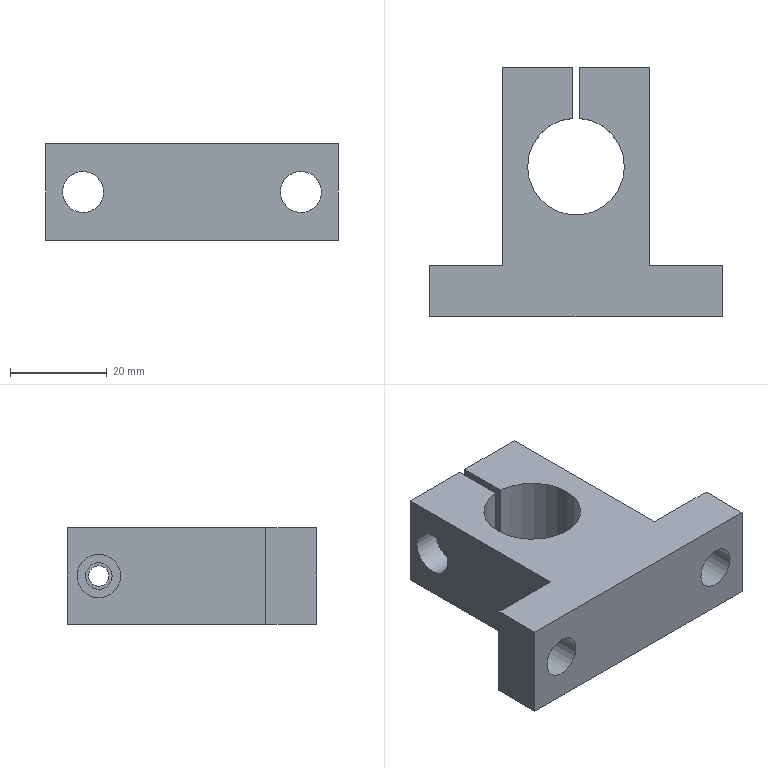Part | STEP file | 20310 | 1 solid | 27 faces | box 60.5 x 51.5 x 20 mm | volume 29160 mm3 | plane 14 | cylinder 13 | commonest cylinder face diameters 8.5 x4 20 x3 4.2 x2 5.5 x2 9 x2
STEP:
#1=CARTESIAN_POINT('',(-26.23,0.,7.962));
#2=VERTEX_POINT('',#1);
#3=CARTESIAN_POINT('',(-26.23,10.5,7.962));
#4=VERTEX_POINT('',#3);
#5=CARTESIAN_POINT('',(-26.23,13.155,7.962));
#6=DIRECTION('',(0.,-1.,0.));
#7=VECTOR('',#6,1.);
#8=LINE('',#5,#7);
#9=EDGE_CURVE('',#2,#4,#8,.F.);
#10=ORIENTED_EDGE('',*,*,#9,.F.);
#11=CARTESIAN_POINT('',(-18.77,0.,12.038));
#12=VERTEX_POINT('',#11);
#13=CARTESIAN_POINT('',(-22.5,0.,10.));
#14=DIRECTION('',(0.,-1.,0.));
#15=AXIS2_PLACEMENT_3D('',#13,#14,$);
#16=CIRCLE('',#15,4.25);
#17=EDGE_CURVE('',#12,#2,#16,.F.);
#18=ORIENTED_EDGE('',*,*,#17,.F.);
#19=CARTESIAN_POINT('',(-18.77,10.5,12.038));
#20=VERTEX_POINT('',#19);
#21=CARTESIAN_POINT('',(-18.77,13.155,12.038));
#22=DIRECTION('',(0.,-1.,0.));
#23=VECTOR('',#22,1.);
#24=LINE('',#21,#23);
#25=EDGE_CURVE('',#12,#20,#24,.F.);
#26=ORIENTED_EDGE('',*,*,#25,.T.);
#27=CARTESIAN_POINT('',(-22.5,10.5,10.));
#28=DIRECTION('',(0.,-1.,0.));
#29=AXIS2_PLACEMENT_3D('',#27,#28,$);
#30=CIRCLE('',#29,4.25);
#31=EDGE_CURVE('',#4,#20,#30,.T.);
#32=ORIENTED_EDGE('',*,*,#31,.F.);
#33=EDGE_LOOP('',(#10,#18,#26,#32));
#34=FACE_OUTER_BOUND('',#33,.T.);
#35=CARTESIAN_POINT('',(-22.5,10.4,10.));
#36=DIRECTION('',(0.,-1.,0.));
#37=DIRECTION('',(0.8776,0.,0.4794));
#38=AXIS2_PLACEMENT_3D('',#35,#36,#37);
#39=CYLINDRICAL_SURFACE('',#38,4.25);
#40=ADVANCED_FACE('',(#34),#39,.F.);
#41=ORIENTED_EDGE('',*,*,#25,.F.);
#42=CARTESIAN_POINT('',(-22.5,0.,10.));
#43=DIRECTION('',(0.,-1.,0.));
#44=AXIS2_PLACEMENT_3D('',#42,#43,$);
#45=CIRCLE('',#44,4.25);
#46=EDGE_CURVE('',#2,#12,#45,.F.);
#47=ORIENTED_EDGE('',*,*,#46,.F.);
#48=ORIENTED_EDGE('',*,*,#9,.T.);
#49=CARTESIAN_POINT('',(-22.5,10.5,10.));
#50=DIRECTION('',(0.,-1.,0.));
#51=AXIS2_PLACEMENT_3D('',#49,#50,$);
#52=CIRCLE('',#51,4.25);
#53=EDGE_CURVE('',#20,#4,#52,.T.);
#54=ORIENTED_EDGE('',*,*,#53,.F.);
#55=EDGE_LOOP('',(#41,#47,#48,#54));
#56=FACE_OUTER_BOUND('',#55,.T.);
#57=ADVANCED_FACE('',(#56),#39,.F.);
#58=CARTESIAN_POINT('',(-30.25,10.5,0.));
#59=VERTEX_POINT('',#58);
#60=CARTESIAN_POINT('',(-30.25,10.5,20.));
#61=VERTEX_POINT('',#60);
#62=CARTESIAN_POINT('',(-30.25,10.5,10.));
#63=DIRECTION('',(0.,0.,1.));
#64=VECTOR('',#63,1.);
#65=LINE('',#62,#64);
#66=EDGE_CURVE('',#59,#61,#65,.T.);
#67=ORIENTED_EDGE('',*,*,#66,.F.);
#68=CARTESIAN_POINT('',(-30.25,0.,0.));
#69=VERTEX_POINT('',#68);
#70=CARTESIAN_POINT('',(-30.25,5.25,0.));
#71=DIRECTION('',(0.,1.,0.));
#72=VECTOR('',#71,1.);
#73=LINE('',#70,#72);
#74=EDGE_CURVE('',#59,#69,#73,.F.);
#75=ORIENTED_EDGE('',*,*,#74,.T.);
#76=CARTESIAN_POINT('',(-30.25,0.,20.));
#77=VERTEX_POINT('',#76);
#78=CARTESIAN_POINT('',(-30.25,0.,10.));
#79=DIRECTION('',(0.,0.,1.));
#80=VECTOR('',#79,1.);
#81=LINE('',#78,#80);
#82=EDGE_CURVE('',#69,#77,#81,.T.);
#83=ORIENTED_EDGE('',*,*,#82,.T.);
#84=CARTESIAN_POINT('',(-30.25,5.25,20.));
#85=DIRECTION('',(0.,1.,0.));
#86=VECTOR('',#85,1.);
#87=LINE('',#84,#86);
#88=EDGE_CURVE('',#61,#77,#87,.F.);
#89=ORIENTED_EDGE('',*,*,#88,.F.);
#90=EDGE_LOOP('',(#67,#75,#83,#89));
#91=FACE_OUTER_BOUND('',#90,.T.);
#92=CARTESIAN_POINT('',(-30.25,0.,0.));
#93=DIRECTION('',(1.,0.,0.));
#94=DIRECTION('',(0.,1.,0.));
#95=AXIS2_PLACEMENT_3D('',#92,#93,#94);
#96=PLANE('',#95);
#97=ADVANCED_FACE('',(#91),#96,.F.);
#98=CARTESIAN_POINT('',(-0.75,51.5,0.));
#99=VERTEX_POINT('',#98);
#100=CARTESIAN_POINT('',(-0.75,40.972,0.));
#101=VERTEX_POINT('',#100);
#102=CARTESIAN_POINT('',(-0.75,46.236,0.));
#103=DIRECTION('',(0.,1.,0.));
#104=VECTOR('',#103,1.);
#105=LINE('',#102,#104);
#106=EDGE_CURVE('',#99,#101,#105,.F.);
#107=ORIENTED_EDGE('',*,*,#106,.T.);
#108=CARTESIAN_POINT('',(-10.,31.,0.));
#109=VERTEX_POINT('',#108);
#110=CARTESIAN_POINT('',(0.,31.,0.));
#111=DIRECTION('',(0.,0.,1.));
#112=AXIS2_PLACEMENT_3D('',#110,#111,$);
#113=CIRCLE('',#112,10.);
#114=EDGE_CURVE('',#101,#109,#113,.T.);
#115=ORIENTED_EDGE('',*,*,#114,.T.);
#116=CARTESIAN_POINT('',(10.,31.,0.));
#117=VERTEX_POINT('',#116);
#118=CARTESIAN_POINT('',(0.,31.,0.));
#119=DIRECTION('',(0.,0.,1.));
#120=AXIS2_PLACEMENT_3D('',#118,#119,$);
#121=CIRCLE('',#120,10.);
#122=EDGE_CURVE('',#109,#117,#121,.T.);
#123=ORIENTED_EDGE('',*,*,#122,.T.);
#124=CARTESIAN_POINT('',(0.75,40.972,0.));
#125=VERTEX_POINT('',#124);
#126=CARTESIAN_POINT('',(0.,31.,0.));
#127=DIRECTION('',(0.,0.,1.));
#128=AXIS2_PLACEMENT_3D('',#126,#127,$);
#129=CIRCLE('',#128,10.);
#130=EDGE_CURVE('',#117,#125,#129,.T.);
#131=ORIENTED_EDGE('',*,*,#130,.T.);
#132=CARTESIAN_POINT('',(0.75,51.5,0.));
#133=VERTEX_POINT('',#132);
#134=CARTESIAN_POINT('',(0.75,46.236,0.));
#135=DIRECTION('',(0.,-1.,0.));
#136=VECTOR('',#135,1.);
#137=LINE('',#134,#136);
#138=EDGE_CURVE('',#125,#133,#137,.F.);
#139=ORIENTED_EDGE('',*,*,#138,.T.);
#140=CARTESIAN_POINT('',(15.25,51.5,0.));
#141=VERTEX_POINT('',#140);
#142=CARTESIAN_POINT('',(8.,51.5,0.));
#143=DIRECTION('',(1.,0.,0.));
#144=VECTOR('',#143,1.);
#145=LINE('',#142,#144);
#146=EDGE_CURVE('',#141,#133,#145,.F.);
#147=ORIENTED_EDGE('',*,*,#146,.F.);
#148=CARTESIAN_POINT('',(15.25,10.5,0.));
#149=VERTEX_POINT('',#148);
#150=CARTESIAN_POINT('',(15.25,31.,0.));
#151=DIRECTION('',(0.,-1.,0.));
#152=VECTOR('',#151,1.);
#153=LINE('',#150,#152);
#154=EDGE_CURVE('',#149,#141,#153,.F.);
#155=ORIENTED_EDGE('',*,*,#154,.F.);
#156=CARTESIAN_POINT('',(30.25,10.5,0.));
#157=VERTEX_POINT('',#156);
#158=CARTESIAN_POINT('',(22.75,10.5,0.));
#159=DIRECTION('',(1.,0.,0.));
#160=VECTOR('',#159,1.);
#161=LINE('',#158,#160);
#162=EDGE_CURVE('',#157,#149,#161,.F.);
#163=ORIENTED_EDGE('',*,*,#162,.F.);
#164=CARTESIAN_POINT('',(30.25,0.,0.));
#165=VERTEX_POINT('',#164);
#166=CARTESIAN_POINT('',(30.25,5.25,0.));
#167=DIRECTION('',(0.,-1.,0.));
#168=VECTOR('',#167,1.);
#169=LINE('',#166,#168);
#170=EDGE_CURVE('',#165,#157,#169,.F.);
#171=ORIENTED_EDGE('',*,*,#170,.F.);
#172=CARTESIAN_POINT('',(0.,0.,0.));
#173=DIRECTION('',(-1.,0.,0.));
#174=VECTOR('',#173,1.);
#175=LINE('',#172,#174);
#176=EDGE_CURVE('',#69,#165,#175,.F.);
#177=ORIENTED_EDGE('',*,*,#176,.F.);
#178=ORIENTED_EDGE('',*,*,#74,.F.);
#179=CARTESIAN_POINT('',(-15.25,10.5,0.));
#180=VERTEX_POINT('',#179);
#181=CARTESIAN_POINT('',(-22.75,10.5,0.));
#182=DIRECTION('',(1.,0.,0.));
#183=VECTOR('',#182,1.);
#184=LINE('',#181,#183);
#185=EDGE_CURVE('',#180,#59,#184,.F.);
#186=ORIENTED_EDGE('',*,*,#185,.F.);
#187=CARTESIAN_POINT('',(-15.25,51.5,0.));
#188=VERTEX_POINT('',#187);
#189=CARTESIAN_POINT('',(-15.25,31.,0.));
#190=DIRECTION('',(0.,1.,0.));
#191=VECTOR('',#190,1.);
#192=LINE('',#189,#191);
#193=EDGE_CURVE('',#188,#180,#192,.F.);
#194=ORIENTED_EDGE('',*,*,#193,.F.);
#195=CARTESIAN_POINT('',(-8.,51.5,0.));
#196=DIRECTION('',(1.,0.,0.));
#197=VECTOR('',#196,1.);
#198=LINE('',#195,#197);
#199=EDGE_CURVE('',#99,#188,#198,.F.);
#200=ORIENTED_EDGE('',*,*,#199,.F.);
#201=EDGE_LOOP('',(#107,#115,#123,#131,#139,#147,#155,#163,#171,#177,#178,#186,#194,#200));
#202=FACE_OUTER_BOUND('',#201,.T.);
#203=CARTESIAN_POINT('',(0.,0.,0.));
#204=DIRECTION('',(0.,0.,1.));
#205=DIRECTION('',(1.,0.,0.));
#206=AXIS2_PLACEMENT_3D('',#203,#204,#205);
#207=PLANE('',#206);
#208=ADVANCED_FACE('',(#202),#207,.F.);
#209=ORIENTED_EDGE('',*,*,#138,.F.);
#210=CARTESIAN_POINT('',(0.75,40.972,20.));
#211=VERTEX_POINT('',#210);
#212=CARTESIAN_POINT('',(0.75,40.972,10.));
#213=DIRECTION('',(0.,0.,1.));
#214=VECTOR('',#213,1.);
#215=LINE('',#212,#214);
#216=EDGE_CURVE('',#125,#211,#215,.T.);
#217=ORIENTED_EDGE('',*,*,#216,.T.);
#218=CARTESIAN_POINT('',(0.75,51.5,20.));
#219=VERTEX_POINT('',#218);
#220=CARTESIAN_POINT('',(0.75,46.236,20.));
#221=DIRECTION('',(0.,-1.,0.));
#222=VECTOR('',#221,1.);
#223=LINE('',#220,#222);
#224=EDGE_CURVE('',#211,#219,#223,.F.);
#225=ORIENTED_EDGE('',*,*,#224,.T.);
#226=CARTESIAN_POINT('',(0.75,51.5,10.));
#227=DIRECTION('',(0.,0.,-1.));
#228=VECTOR('',#227,1.);
#229=LINE('',#226,#228);
#230=EDGE_CURVE('',#219,#133,#229,.T.);
#231=ORIENTED_EDGE('',*,*,#230,.T.);
#232=EDGE_LOOP('',(#209,#217,#225,#231));
#233=FACE_OUTER_BOUND('',#232,.T.);
#234=CARTESIAN_POINT('',(0.75,43.157,8.993));
#235=VERTEX_POINT('',#234);
#236=CARTESIAN_POINT('',(0.75,46.843,11.007));
#237=VERTEX_POINT('',#236);
#238=CARTESIAN_POINT('',(0.75,45.,10.));
#239=DIRECTION('',(1.,0.,0.));
#240=AXIS2_PLACEMENT_3D('',#238,#239,$);
#241=CIRCLE('',#240,2.1);
#242=EDGE_CURVE('',#235,#237,#241,.T.);
#243=ORIENTED_EDGE('',*,*,#242,.T.);
#244=CARTESIAN_POINT('',(0.75,45.,10.));
#245=DIRECTION('',(1.,0.,0.));
#246=AXIS2_PLACEMENT_3D('',#244,#245,$);
#247=CIRCLE('',#246,2.1);
#248=EDGE_CURVE('',#237,#235,#247,.T.);
#249=ORIENTED_EDGE('',*,*,#248,.T.);
#250=EDGE_LOOP('',(#243,#249));
#251=FACE_BOUND('',#250,.T.);
#252=CARTESIAN_POINT('',(0.75,60.,20.));
#253=DIRECTION('',(1.,0.,0.));
#254=DIRECTION('',(0.,-1.,0.));
#255=AXIS2_PLACEMENT_3D('',#252,#253,#254);
#256=PLANE('',#255);
#257=ADVANCED_FACE('',(#233,#251),#256,.F.);
#258=ORIENTED_EDGE('',*,*,#216,.F.);
#259=ORIENTED_EDGE('',*,*,#130,.F.);
#260=CARTESIAN_POINT('',(10.,31.,20.));
#261=VERTEX_POINT('',#260);
#262=CARTESIAN_POINT('',(10.,31.,10.));
#263=DIRECTION('',(0.,0.,1.));
#264=VECTOR('',#263,1.);
#265=LINE('',#262,#264);
#266=EDGE_CURVE('',#261,#117,#265,.F.);
#267=ORIENTED_EDGE('',*,*,#266,.F.);
#268=CARTESIAN_POINT('',(0.,31.,20.));
#269=DIRECTION('',(0.,0.,1.));
#270=AXIS2_PLACEMENT_3D('',#268,#269,$);
#271=CIRCLE('',#270,10.);
#272=EDGE_CURVE('',#261,#211,#271,.T.);
#273=ORIENTED_EDGE('',*,*,#272,.T.);
#274=EDGE_LOOP('',(#258,#259,#267,#273));
#275=FACE_OUTER_BOUND('',#274,.T.);
#276=CARTESIAN_POINT('',(0.,31.,10.));
#277=DIRECTION('',(0.,0.,1.));
#278=DIRECTION('',(1.,0.,0.));
#279=AXIS2_PLACEMENT_3D('',#276,#277,#278);
#280=CYLINDRICAL_SURFACE('',#279,10.);
#281=ADVANCED_FACE('',(#275),#280,.F.);
#282=CARTESIAN_POINT('',(-10.,31.,20.));
#283=VERTEX_POINT('',#282);
#284=CARTESIAN_POINT('',(-10.,31.,10.));
#285=DIRECTION('',(0.,0.,1.));
#286=VECTOR('',#285,1.);
#287=LINE('',#284,#286);
#288=EDGE_CURVE('',#283,#109,#287,.F.);
#289=ORIENTED_EDGE('',*,*,#288,.F.);
#290=CARTESIAN_POINT('',(0.,31.,20.));
#291=DIRECTION('',(0.,0.,1.));
#292=AXIS2_PLACEMENT_3D('',#290,#291,$);
#293=CIRCLE('',#292,10.);
#294=EDGE_CURVE('',#283,#261,#293,.T.);
#295=ORIENTED_EDGE('',*,*,#294,.T.);
#296=ORIENTED_EDGE('',*,*,#266,.T.);
#297=ORIENTED_EDGE('',*,*,#122,.F.);
#298=EDGE_LOOP('',(#289,#295,#296,#297));
#299=FACE_OUTER_BOUND('',#298,.T.);
#300=ADVANCED_FACE('',(#299),#280,.F.);
#301=CARTESIAN_POINT('',(-0.75,40.972,20.));
#302=VERTEX_POINT('',#301);
#303=CARTESIAN_POINT('',(-0.75,40.972,10.));
#304=DIRECTION('',(0.,0.,1.));
#305=VECTOR('',#304,1.);
#306=LINE('',#303,#305);
#307=EDGE_CURVE('',#101,#302,#306,.T.);
#308=ORIENTED_EDGE('',*,*,#307,.T.);
#309=CARTESIAN_POINT('',(0.,31.,20.));
#310=DIRECTION('',(0.,0.,1.));
#311=AXIS2_PLACEMENT_3D('',#309,#310,$);
#312=CIRCLE('',#311,10.);
#313=EDGE_CURVE('',#302,#283,#312,.T.);
#314=ORIENTED_EDGE('',*,*,#313,.T.);
#315=ORIENTED_EDGE('',*,*,#288,.T.);
#316=ORIENTED_EDGE('',*,*,#114,.F.);
#317=EDGE_LOOP('',(#308,#314,#315,#316));
#318=FACE_OUTER_BOUND('',#317,.T.);
#319=ADVANCED_FACE('',(#318),#280,.F.);
#320=ORIENTED_EDGE('',*,*,#106,.F.);
#321=CARTESIAN_POINT('',(-0.75,51.5,20.));
#322=VERTEX_POINT('',#321);
#323=CARTESIAN_POINT('',(-0.75,51.5,10.));
#324=DIRECTION('',(0.,0.,-1.));
#325=VECTOR('',#324,1.);
#326=LINE('',#323,#325);
#327=EDGE_CURVE('',#322,#99,#326,.T.);
#328=ORIENTED_EDGE('',*,*,#327,.F.);
#329=CARTESIAN_POINT('',(-0.75,46.236,20.));
#330=DIRECTION('',(0.,1.,0.));
#331=VECTOR('',#330,1.);
#332=LINE('',#329,#331);
#333=EDGE_CURVE('',#322,#302,#332,.F.);
#334=ORIENTED_EDGE('',*,*,#333,.T.);
#335=ORIENTED_EDGE('',*,*,#307,.F.);
#336=EDGE_LOOP('',(#320,#328,#334,#335));
#337=FACE_OUTER_BOUND('',#336,.T.);
#338=CARTESIAN_POINT('',(-0.75,42.587,8.682));
#339=VERTEX_POINT('',#338);
#340=CARTESIAN_POINT('',(-0.75,47.413,11.318));
#341=VERTEX_POINT('',#340);
#342=CARTESIAN_POINT('',(-0.75,45.,10.));
#343=DIRECTION('',(-1.,0.,0.));
#344=AXIS2_PLACEMENT_3D('',#342,#343,$);
#345=CIRCLE('',#344,2.75);
#346=EDGE_CURVE('',#339,#341,#345,.T.);
#347=ORIENTED_EDGE('',*,*,#346,.T.);
#348=CARTESIAN_POINT('',(-0.75,45.,10.));
#349=DIRECTION('',(-1.,0.,0.));
#350=AXIS2_PLACEMENT_3D('',#348,#349,$);
#351=CIRCLE('',#350,2.75);
#352=EDGE_CURVE('',#341,#339,#351,.T.);
#353=ORIENTED_EDGE('',*,*,#352,.T.);
#354=EDGE_LOOP('',(#347,#353));
#355=FACE_BOUND('',#354,.T.);
#356=CARTESIAN_POINT('',(-0.75,30.,20.));
#357=DIRECTION('',(-1.,0.,0.));
#358=DIRECTION('',(0.,1.,0.));
#359=AXIS2_PLACEMENT_3D('',#356,#357,#358);
#360=PLANE('',#359);
#361=ADVANCED_FACE('',(#337,#355),#360,.F.);
#362=CARTESIAN_POINT('',(15.25,46.843,11.007));
#363=VERTEX_POINT('',#362);
#364=CARTESIAN_POINT('',(-4.905,46.843,11.007));
#365=DIRECTION('',(1.,0.,0.));
#366=VECTOR('',#365,1.);
#367=LINE('',#364,#366);
#368=EDGE_CURVE('',#363,#237,#367,.F.);
#369=ORIENTED_EDGE('',*,*,#368,.F.);
#370=CARTESIAN_POINT('',(15.25,43.157,8.993));
#371=VERTEX_POINT('',#370);
#372=CARTESIAN_POINT('',(15.25,45.,10.));
#373=DIRECTION('',(1.,0.,0.));
#374=AXIS2_PLACEMENT_3D('',#372,#373,$);
#375=CIRCLE('',#374,2.1);
#376=EDGE_CURVE('',#371,#363,#375,.F.);
#377=ORIENTED_EDGE('',*,*,#376,.F.);
#378=CARTESIAN_POINT('',(-4.905,43.157,8.993));
#379=DIRECTION('',(1.,0.,0.));
#380=VECTOR('',#379,1.);
#381=LINE('',#378,#380);
#382=EDGE_CURVE('',#371,#235,#381,.F.);
#383=ORIENTED_EDGE('',*,*,#382,.T.);
#384=ORIENTED_EDGE('',*,*,#248,.F.);
#385=EDGE_LOOP('',(#369,#377,#383,#384));
#386=FACE_OUTER_BOUND('',#385,.T.);
#387=CARTESIAN_POINT('',(-15.15,45.,10.));
#388=DIRECTION('',(1.,0.,0.));
#389=DIRECTION('',(0.,0.8776,0.4794));
#390=AXIS2_PLACEMENT_3D('',#387,#388,#389);
#391=CYLINDRICAL_SURFACE('',#390,2.1);
#392=ADVANCED_FACE('',(#386),#391,.F.);
#393=ORIENTED_EDGE('',*,*,#382,.F.);
#394=CARTESIAN_POINT('',(15.25,45.,10.));
#395=DIRECTION('',(1.,0.,0.));
#396=AXIS2_PLACEMENT_3D('',#394,#395,$);
#397=CIRCLE('',#396,2.1);
#398=EDGE_CURVE('',#363,#371,#397,.F.);
#399=ORIENTED_EDGE('',*,*,#398,.F.);
#400=ORIENTED_EDGE('',*,*,#368,.T.);
#401=ORIENTED_EDGE('',*,*,#242,.F.);
#402=EDGE_LOOP('',(#393,#399,#400,#401));
#403=FACE_OUTER_BOUND('',#402,.T.);
#404=ADVANCED_FACE('',(#403),#391,.F.);
#405=ORIENTED_EDGE('',*,*,#352,.F.);
#406=CARTESIAN_POINT('',(-9.75,47.413,11.318));
#407=VERTEX_POINT('',#406);
#408=CARTESIAN_POINT('',(-15.455,47.413,11.318));
#409=DIRECTION('',(1.,0.,0.));
#410=VECTOR('',#409,1.);
#411=LINE('',#408,#410);
#412=EDGE_CURVE('',#341,#407,#411,.F.);
#413=ORIENTED_EDGE('',*,*,#412,.T.);
#414=CARTESIAN_POINT('',(-9.75,42.587,8.682));
#415=VERTEX_POINT('',#414);
#416=CARTESIAN_POINT('',(-9.75,45.,10.));
#417=DIRECTION('',(1.,0.,0.));
#418=AXIS2_PLACEMENT_3D('',#416,#417,$);
#419=CIRCLE('',#418,2.75);
#420=EDGE_CURVE('',#415,#407,#419,.T.);
#421=ORIENTED_EDGE('',*,*,#420,.F.);
#422=CARTESIAN_POINT('',(-15.455,42.587,8.682));
#423=DIRECTION('',(1.,0.,0.));
#424=VECTOR('',#423,1.);
#425=LINE('',#422,#424);
#426=EDGE_CURVE('',#339,#415,#425,.F.);
#427=ORIENTED_EDGE('',*,*,#426,.F.);
#428=EDGE_LOOP('',(#405,#413,#421,#427));
#429=FACE_OUTER_BOUND('',#428,.T.);
#430=CARTESIAN_POINT('',(-15.15,45.,10.));
#431=DIRECTION('',(1.,0.,0.));
#432=DIRECTION('',(0.,0.8776,0.4794));
#433=AXIS2_PLACEMENT_3D('',#430,#431,#432);
#434=CYLINDRICAL_SURFACE('',#433,2.75);
#435=ADVANCED_FACE('',(#429),#434,.F.);
#436=ORIENTED_EDGE('',*,*,#346,.F.);
#437=ORIENTED_EDGE('',*,*,#426,.T.);
#438=CARTESIAN_POINT('',(-9.75,45.,10.));
#439=DIRECTION('',(1.,0.,0.));
#440=AXIS2_PLACEMENT_3D('',#438,#439,$);
#441=CIRCLE('',#440,2.75);
#442=EDGE_CURVE('',#407,#415,#441,.T.);
#443=ORIENTED_EDGE('',*,*,#442,.F.);
#444=ORIENTED_EDGE('',*,*,#412,.F.);
#445=EDGE_LOOP('',(#436,#437,#443,#444));
#446=FACE_OUTER_BOUND('',#445,.T.);
#447=ADVANCED_FACE('',(#446),#434,.F.);
#448=CARTESIAN_POINT('',(-15.25,48.949,12.157));
#449=VERTEX_POINT('',#448);
#450=CARTESIAN_POINT('',(-15.25,41.051,7.843));
#451=VERTEX_POINT('',#450);
#452=CARTESIAN_POINT('',(-15.25,45.,10.));
#453=DIRECTION('',(1.,0.,0.));
#454=AXIS2_PLACEMENT_3D('',#452,#453,$);
#455=CIRCLE('',#454,4.5);
#456=EDGE_CURVE('',#449,#451,#455,.T.);
#457=ORIENTED_EDGE('',*,*,#456,.F.);
#458=CARTESIAN_POINT('',(-9.75,48.949,12.157));
#459=VERTEX_POINT('',#458);
#460=CARTESIAN_POINT('',(-20.155,48.949,12.157));
#461=DIRECTION('',(1.,0.,0.));
#462=VECTOR('',#461,1.);
#463=LINE('',#460,#462);
#464=EDGE_CURVE('',#459,#449,#463,.F.);
#465=ORIENTED_EDGE('',*,*,#464,.F.);
#466=CARTESIAN_POINT('',(-9.75,41.051,7.843));
#467=VERTEX_POINT('',#466);
#468=CARTESIAN_POINT('',(-9.75,45.,10.));
#469=DIRECTION('',(1.,0.,0.));
#470=AXIS2_PLACEMENT_3D('',#468,#469,$);
#471=CIRCLE('',#470,4.5);
#472=EDGE_CURVE('',#459,#467,#471,.T.);
#473=ORIENTED_EDGE('',*,*,#472,.T.);
#474=CARTESIAN_POINT('',(-20.155,41.051,7.843));
#475=DIRECTION('',(1.,0.,0.));
#476=VECTOR('',#475,1.);
#477=LINE('',#474,#476);
#478=EDGE_CURVE('',#467,#451,#477,.F.);
#479=ORIENTED_EDGE('',*,*,#478,.T.);
#480=EDGE_LOOP('',(#457,#465,#473,#479));
#481=FACE_OUTER_BOUND('',#480,.T.);
#482=CARTESIAN_POINT('',(-15.15,45.,10.));
#483=DIRECTION('',(1.,0.,0.));
#484=DIRECTION('',(0.,0.8776,0.4794));
#485=AXIS2_PLACEMENT_3D('',#482,#483,#484);
#486=CYLINDRICAL_SURFACE('',#485,4.5);
#487=ADVANCED_FACE('',(#481),#486,.F.);
#488=CARTESIAN_POINT('',(-15.25,45.,10.));
#489=DIRECTION('',(1.,0.,0.));
#490=AXIS2_PLACEMENT_3D('',#488,#489,$);
#491=CIRCLE('',#490,4.5);
#492=EDGE_CURVE('',#451,#449,#491,.T.);
#493=ORIENTED_EDGE('',*,*,#492,.F.);
#494=ORIENTED_EDGE('',*,*,#478,.F.);
#495=CARTESIAN_POINT('',(-9.75,45.,10.));
#496=DIRECTION('',(1.,0.,0.));
#497=AXIS2_PLACEMENT_3D('',#495,#496,$);
#498=CIRCLE('',#497,4.5);
#499=EDGE_CURVE('',#467,#459,#498,.T.);
#500=ORIENTED_EDGE('',*,*,#499,.T.);
#501=ORIENTED_EDGE('',*,*,#464,.T.);
#502=EDGE_LOOP('',(#493,#494,#500,#501));
#503=FACE_OUTER_BOUND('',#502,.T.);
#504=ADVANCED_FACE('',(#503),#486,.F.);
#505=ORIENTED_EDGE('',*,*,#472,.F.);
#506=ORIENTED_EDGE('',*,*,#499,.F.);
#507=EDGE_LOOP('',(#505,#506));
#508=FACE_OUTER_BOUND('',#507,.T.);
#509=ORIENTED_EDGE('',*,*,#420,.T.);
#510=ORIENTED_EDGE('',*,*,#442,.T.);
#511=EDGE_LOOP('',(#509,#510));
#512=FACE_BOUND('',#511,.T.);
#513=CARTESIAN_POINT('',(-9.75,47.75,10.));
#514=DIRECTION('',(1.,0.,0.));
#515=DIRECTION('',(0.,1.,0.));
#516=AXIS2_PLACEMENT_3D('',#513,#514,#515);
#517=PLANE('',#516);
#518=ADVANCED_FACE('',(#508,#512),#517,.F.);
#519=ORIENTED_EDGE('',*,*,#230,.F.);
#520=CARTESIAN_POINT('',(15.25,51.5,20.));
#521=VERTEX_POINT('',#520);
#522=CARTESIAN_POINT('',(8.,51.5,20.));
#523=DIRECTION('',(1.,0.,0.));
#524=VECTOR('',#523,1.);
#525=LINE('',#522,#524);
#526=EDGE_CURVE('',#521,#219,#525,.F.);
#527=ORIENTED_EDGE('',*,*,#526,.F.);
#528=CARTESIAN_POINT('',(15.25,51.5,10.));
#529=DIRECTION('',(0.,0.,1.));
#530=VECTOR('',#529,1.);
#531=LINE('',#528,#530);
#532=EDGE_CURVE('',#141,#521,#531,.T.);
#533=ORIENTED_EDGE('',*,*,#532,.F.);
#534=ORIENTED_EDGE('',*,*,#146,.T.);
#535=EDGE_LOOP('',(#519,#527,#533,#534));
#536=FACE_OUTER_BOUND('',#535,.T.);
#537=CARTESIAN_POINT('',(-15.25,51.5,0.));
#538=DIRECTION('',(0.,-1.,0.));
#539=DIRECTION('',(1.,0.,0.));
#540=AXIS2_PLACEMENT_3D('',#537,#538,#539);
#541=PLANE('',#540);
#542=ADVANCED_FACE('',(#536),#541,.F.);
#543=CARTESIAN_POINT('',(15.25,10.5,20.));
#544=VERTEX_POINT('',#543);
#545=CARTESIAN_POINT('',(15.25,10.5,10.));
#546=DIRECTION('',(0.,0.,1.));
#547=VECTOR('',#546,1.);
#548=LINE('',#545,#547);
#549=EDGE_CURVE('',#149,#544,#548,.T.);
#550=ORIENTED_EDGE('',*,*,#549,.F.);
#551=ORIENTED_EDGE('',*,*,#154,.T.);
#552=ORIENTED_EDGE('',*,*,#532,.T.);
#553=CARTESIAN_POINT('',(15.25,31.,20.));
#554=DIRECTION('',(0.,-1.,0.));
#555=VECTOR('',#554,1.);
#556=LINE('',#553,#555);
#557=EDGE_CURVE('',#544,#521,#556,.F.);
#558=ORIENTED_EDGE('',*,*,#557,.F.);
#559=EDGE_LOOP('',(#550,#551,#552,#558));
#560=FACE_OUTER_BOUND('',#559,.T.);
#561=ORIENTED_EDGE('',*,*,#398,.T.);
#562=ORIENTED_EDGE('',*,*,#376,.T.);
#563=EDGE_LOOP('',(#561,#562));
#564=FACE_BOUND('',#563,.T.);
#565=CARTESIAN_POINT('',(15.25,51.5,0.));
#566=DIRECTION('',(-1.,0.,0.));
#567=DIRECTION('',(0.,-1.,0.));
#568=AXIS2_PLACEMENT_3D('',#565,#566,#567);
#569=PLANE('',#568);
#570=ADVANCED_FACE('',(#560,#564),#569,.F.);
#571=CARTESIAN_POINT('',(30.25,0.,20.));
#572=VERTEX_POINT('',#571);
#573=CARTESIAN_POINT('',(30.25,0.,10.));
#574=DIRECTION('',(0.,0.,1.));
#575=VECTOR('',#574,1.);
#576=LINE('',#573,#575);
#577=EDGE_CURVE('',#165,#572,#576,.T.);
#578=ORIENTED_EDGE('',*,*,#577,.F.);
#579=ORIENTED_EDGE('',*,*,#170,.T.);
#580=CARTESIAN_POINT('',(30.25,10.5,20.));
#581=VERTEX_POINT('',#580);
#582=CARTESIAN_POINT('',(30.25,10.5,10.));
#583=DIRECTION('',(0.,0.,1.));
#584=VECTOR('',#583,1.);
#585=LINE('',#582,#584);
#586=EDGE_CURVE('',#157,#581,#585,.T.);
#587=ORIENTED_EDGE('',*,*,#586,.T.);
#588=CARTESIAN_POINT('',(30.25,5.25,20.));
#589=DIRECTION('',(0.,-1.,0.));
#590=VECTOR('',#589,1.);
#591=LINE('',#588,#590);
#592=EDGE_CURVE('',#572,#581,#591,.F.);
#593=ORIENTED_EDGE('',*,*,#592,.F.);
#594=EDGE_LOOP('',(#578,#579,#587,#593));
#595=FACE_OUTER_BOUND('',#594,.T.);
#596=CARTESIAN_POINT('',(30.25,10.5,0.));
#597=DIRECTION('',(-1.,0.,0.));
#598=DIRECTION('',(0.,-1.,0.));
#599=AXIS2_PLACEMENT_3D('',#596,#597,#598);
#600=PLANE('',#599);
#601=ADVANCED_FACE('',(#595),#600,.F.);
#602=ORIENTED_EDGE('',*,*,#327,.T.);
#603=ORIENTED_EDGE('',*,*,#199,.T.);
#604=CARTESIAN_POINT('',(-15.25,51.5,20.));
#605=VERTEX_POINT('',#604);
#606=CARTESIAN_POINT('',(-15.25,51.5,10.));
#607=DIRECTION('',(0.,0.,1.));
#608=VECTOR('',#607,1.);
#609=LINE('',#606,#608);
#610=EDGE_CURVE('',#188,#605,#609,.T.);
#611=ORIENTED_EDGE('',*,*,#610,.T.);
#612=CARTESIAN_POINT('',(-8.,51.5,20.));
#613=DIRECTION('',(1.,0.,0.));
#614=VECTOR('',#613,1.);
#615=LINE('',#612,#614);
#616=EDGE_CURVE('',#322,#605,#615,.F.);
#617=ORIENTED_EDGE('',*,*,#616,.F.);
#618=EDGE_LOOP('',(#602,#603,#611,#617));
#619=FACE_OUTER_BOUND('',#618,.T.);
#620=ADVANCED_FACE('',(#619),#541,.F.);
#621=ORIENTED_EDGE('',*,*,#610,.F.);
#622=ORIENTED_EDGE('',*,*,#193,.T.);
#623=CARTESIAN_POINT('',(-15.25,10.5,20.));
#624=VERTEX_POINT('',#623);
#625=CARTESIAN_POINT('',(-15.25,10.5,10.));
#626=DIRECTION('',(0.,0.,1.));
#627=VECTOR('',#626,1.);
#628=LINE('',#625,#627);
#629=EDGE_CURVE('',#180,#624,#628,.T.);
#630=ORIENTED_EDGE('',*,*,#629,.T.);
#631=CARTESIAN_POINT('',(-15.25,31.,20.));
#632=DIRECTION('',(0.,1.,0.));
#633=VECTOR('',#632,1.);
#634=LINE('',#631,#633);
#635=EDGE_CURVE('',#605,#624,#634,.F.);
#636=ORIENTED_EDGE('',*,*,#635,.F.);
#637=EDGE_LOOP('',(#621,#622,#630,#636));
#638=FACE_OUTER_BOUND('',#637,.T.);
#639=ORIENTED_EDGE('',*,*,#492,.T.);
#640=ORIENTED_EDGE('',*,*,#456,.T.);
#641=EDGE_LOOP('',(#639,#640));
#642=FACE_BOUND('',#641,.T.);
#643=CARTESIAN_POINT('',(-15.25,10.5,0.));
#644=DIRECTION('',(1.,0.,0.));
#645=DIRECTION('',(0.,1.,0.));
#646=AXIS2_PLACEMENT_3D('',#643,#644,#645);
#647=PLANE('',#646);
#648=ADVANCED_FACE('',(#638,#642),#647,.F.);
#649=ORIENTED_EDGE('',*,*,#616,.T.);
#650=ORIENTED_EDGE('',*,*,#635,.T.);
#651=CARTESIAN_POINT('',(-22.75,10.5,20.));
#652=DIRECTION('',(1.,0.,0.));
#653=VECTOR('',#652,1.);
#654=LINE('',#651,#653);
#655=EDGE_CURVE('',#624,#61,#654,.F.);
#656=ORIENTED_EDGE('',*,*,#655,.T.);
#657=ORIENTED_EDGE('',*,*,#88,.T.);
#658=CARTESIAN_POINT('',(0.,0.,20.));
#659=DIRECTION('',(-1.,0.,0.));
#660=VECTOR('',#659,1.);
#661=LINE('',#658,#660);
#662=EDGE_CURVE('',#77,#572,#661,.F.);
#663=ORIENTED_EDGE('',*,*,#662,.T.);
#664=ORIENTED_EDGE('',*,*,#592,.T.);
#665=CARTESIAN_POINT('',(22.75,10.5,20.));
#666=DIRECTION('',(1.,0.,0.));
#667=VECTOR('',#666,1.);
#668=LINE('',#665,#667);
#669=EDGE_CURVE('',#581,#544,#668,.F.);
#670=ORIENTED_EDGE('',*,*,#669,.T.);
#671=ORIENTED_EDGE('',*,*,#557,.T.);
#672=ORIENTED_EDGE('',*,*,#526,.T.);
#673=ORIENTED_EDGE('',*,*,#224,.F.);
#674=ORIENTED_EDGE('',*,*,#272,.F.);
#675=ORIENTED_EDGE('',*,*,#294,.F.);
#676=ORIENTED_EDGE('',*,*,#313,.F.);
#677=ORIENTED_EDGE('',*,*,#333,.F.);
#678=EDGE_LOOP('',(#649,#650,#656,#657,#663,#664,#670,#671,#672,#673,#674,#675,#676,#677));
#679=FACE_OUTER_BOUND('',#678,.T.);
#680=CARTESIAN_POINT('',(0.,0.,20.));
#681=DIRECTION('',(0.,0.,1.));
#682=DIRECTION('',(1.,0.,0.));
#683=AXIS2_PLACEMENT_3D('',#680,#681,#682);
#684=PLANE('',#683);
#685=ADVANCED_FACE('',(#679),#684,.T.);
#686=ORIENTED_EDGE('',*,*,#629,.F.);
#687=ORIENTED_EDGE('',*,*,#185,.T.);
#688=ORIENTED_EDGE('',*,*,#66,.T.);
#689=ORIENTED_EDGE('',*,*,#655,.F.);
#690=EDGE_LOOP('',(#686,#687,#688,#689));
#691=FACE_OUTER_BOUND('',#690,.T.);
#692=ORIENTED_EDGE('',*,*,#31,.T.);
#693=ORIENTED_EDGE('',*,*,#53,.T.);
#694=EDGE_LOOP('',(#692,#693));
#695=FACE_BOUND('',#694,.T.);
#696=CARTESIAN_POINT('',(-30.25,10.5,0.));
#697=DIRECTION('',(0.,-1.,0.));
#698=DIRECTION('',(1.,0.,0.));
#699=AXIS2_PLACEMENT_3D('',#696,#697,#698);
#700=PLANE('',#699);
#701=ADVANCED_FACE('',(#691,#695),#700,.F.);
#702=ORIENTED_EDGE('',*,*,#82,.F.);
#703=ORIENTED_EDGE('',*,*,#176,.T.);
#704=ORIENTED_EDGE('',*,*,#577,.T.);
#705=ORIENTED_EDGE('',*,*,#662,.F.);
#706=EDGE_LOOP('',(#702,#703,#704,#705));
#707=FACE_OUTER_BOUND('',#706,.T.);
#708=CARTESIAN_POINT('',(26.23,0.,12.038));
#709=VERTEX_POINT('',#708);
#710=CARTESIAN_POINT('',(18.77,0.,7.962));
#711=VERTEX_POINT('',#710);
#712=CARTESIAN_POINT('',(22.5,0.,10.));
#713=DIRECTION('',(0.,1.,0.));
#714=AXIS2_PLACEMENT_3D('',#712,#713,$);
#715=CIRCLE('',#714,4.25);
#716=EDGE_CURVE('',#709,#711,#715,.T.);
#717=ORIENTED_EDGE('',*,*,#716,.T.);
#718=CARTESIAN_POINT('',(22.5,0.,10.));
#719=DIRECTION('',(0.,1.,0.));
#720=AXIS2_PLACEMENT_3D('',#718,#719,$);
#721=CIRCLE('',#720,4.25);
#722=EDGE_CURVE('',#711,#709,#721,.T.);
#723=ORIENTED_EDGE('',*,*,#722,.T.);
#724=EDGE_LOOP('',(#717,#723));
#725=FACE_BOUND('',#724,.T.);
#726=ORIENTED_EDGE('',*,*,#17,.T.);
#727=ORIENTED_EDGE('',*,*,#46,.T.);
#728=EDGE_LOOP('',(#726,#727));
#729=FACE_BOUND('',#728,.T.);
#730=CARTESIAN_POINT('',(30.25,0.,0.));
#731=DIRECTION('',(0.,1.,0.));
#732=DIRECTION('',(-1.,0.,0.));
#733=AXIS2_PLACEMENT_3D('',#730,#731,#732);
#734=PLANE('',#733);
#735=ADVANCED_FACE('',(#707,#725,#729),#734,.F.);
#736=ORIENTED_EDGE('',*,*,#586,.F.);
#737=ORIENTED_EDGE('',*,*,#162,.T.);
#738=ORIENTED_EDGE('',*,*,#549,.T.);
#739=ORIENTED_EDGE('',*,*,#669,.F.);
#740=EDGE_LOOP('',(#736,#737,#738,#739));
#741=FACE_OUTER_BOUND('',#740,.T.);
#742=CARTESIAN_POINT('',(18.77,10.5,7.962));
#743=VERTEX_POINT('',#742);
#744=CARTESIAN_POINT('',(26.23,10.5,12.038));
#745=VERTEX_POINT('',#744);
#746=CARTESIAN_POINT('',(22.5,10.5,10.));
#747=DIRECTION('',(0.,-1.,0.));
#748=AXIS2_PLACEMENT_3D('',#746,#747,$);
#749=CIRCLE('',#748,4.25);
#750=EDGE_CURVE('',#743,#745,#749,.T.);
#751=ORIENTED_EDGE('',*,*,#750,.T.);
#752=CARTESIAN_POINT('',(22.5,10.5,10.));
#753=DIRECTION('',(0.,-1.,0.));
#754=AXIS2_PLACEMENT_3D('',#752,#753,$);
#755=CIRCLE('',#754,4.25);
#756=EDGE_CURVE('',#745,#743,#755,.T.);
#757=ORIENTED_EDGE('',*,*,#756,.T.);
#758=EDGE_LOOP('',(#751,#757));
#759=FACE_BOUND('',#758,.T.);
#760=ADVANCED_FACE('',(#741,#759),#700,.F.);
#761=CARTESIAN_POINT('',(18.77,13.155,7.962));
#762=DIRECTION('',(0.,-1.,0.));
#763=VECTOR('',#762,1.);
#764=LINE('',#761,#763);
#765=EDGE_CURVE('',#711,#743,#764,.F.);
#766=ORIENTED_EDGE('',*,*,#765,.F.);
#767=ORIENTED_EDGE('',*,*,#716,.F.);
#768=CARTESIAN_POINT('',(26.23,13.155,12.038));
#769=DIRECTION('',(0.,-1.,0.));
#770=VECTOR('',#769,1.);
#771=LINE('',#768,#770);
#772=EDGE_CURVE('',#709,#745,#771,.F.);
#773=ORIENTED_EDGE('',*,*,#772,.T.);
#774=ORIENTED_EDGE('',*,*,#750,.F.);
#775=EDGE_LOOP('',(#766,#767,#773,#774));
#776=FACE_OUTER_BOUND('',#775,.T.);
#777=CARTESIAN_POINT('',(22.5,10.4,10.));
#778=DIRECTION('',(0.,-1.,0.));
#779=DIRECTION('',(0.8776,0.,0.4794));
#780=AXIS2_PLACEMENT_3D('',#777,#778,#779);
#781=CYLINDRICAL_SURFACE('',#780,4.25);
#782=ADVANCED_FACE('',(#776),#781,.F.);
#783=ORIENTED_EDGE('',*,*,#772,.F.);
#784=ORIENTED_EDGE('',*,*,#722,.F.);
#785=ORIENTED_EDGE('',*,*,#765,.T.);
#786=ORIENTED_EDGE('',*,*,#756,.F.);
#787=EDGE_LOOP('',(#783,#784,#785,#786));
#788=FACE_OUTER_BOUND('',#787,.T.);
#789=ADVANCED_FACE('',(#788),#781,.F.);
#790=CLOSED_SHELL('',(#40,#57,#97,#208,#257,#281,#300,#319,#361,#392,#404,#435,#447,#487,#504,#518,#542,#570,#601,#620,#648,#685,#701,#735,#760,#782,#789));
#791=MANIFOLD_SOLID_BREP('',#790);
#792=(LENGTH_UNIT()NAMED_UNIT(*)SI_UNIT(.MILLI.,.METRE.));
#793=UNCERTAINTY_MEASURE_WITH_UNIT(LENGTH_MEASURE(0.005),#792,'','');
#794=(NAMED_UNIT(*)PLANE_ANGLE_UNIT()SI_UNIT($,.RADIAN.));
#795=(NAMED_UNIT(*)SI_UNIT($,.STERADIAN.)SOLID_ANGLE_UNIT());
#796=(GEOMETRIC_REPRESENTATION_CONTEXT(3)GLOBAL_UNCERTAINTY_ASSIGNED_CONTEXT((#793))GLOBAL_UNIT_ASSIGNED_CONTEXT((#792,#794,#795))REPRESENTATION_CONTEXT('',''));
#797=ADVANCED_BREP_SHAPE_REPRESENTATION('',(#791),#796);